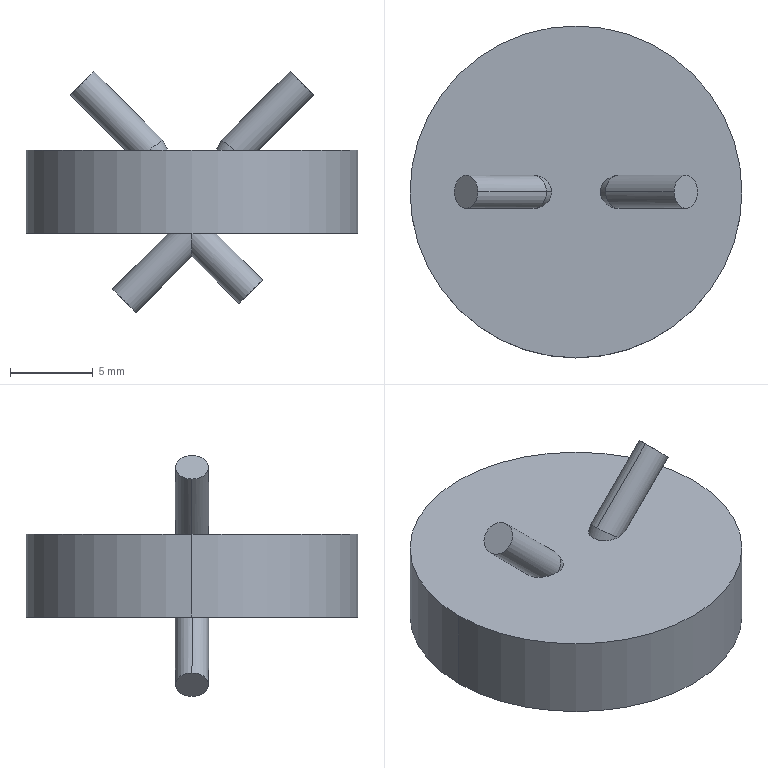Part | SolidWorks | features Sweep 2, Extrusion 1, MirrorPattern 1 | 1 solid | 19 faces | box 20 x 20 x 14.516 mm | volume 1637 mm3 | cylinder 13 | plane 6 | commonest cylinder face diameters 2 x11 20 x2
STEP:
#1=CARTESIAN_POINT('',(1.779,0.,3.098));
#2=VERTEX_POINT('',#1);
#3=CARTESIAN_POINT('',(2.596,1.,2.5));
#4=VERTEX_POINT('',#3);
#5=CARTESIAN_POINT('',(1.779,0.,3.098));
#6=CARTESIAN_POINT('',(1.779,0.5858,3.098));
#7=CARTESIAN_POINT('',(2.118,1.,2.85));
#8=CARTESIAN_POINT('',(2.596,1.,2.5));
#9=(BOUNDED_CURVE()B_SPLINE_CURVE(3,(#5,#6,#7,#8),.UNSPECIFIED.,.F.,.F.)B_SPLINE_CURVE_WITH_KNOTS((4,4),(0.,1.571),.UNSPECIFIED.)CURVE()GEOMETRIC_REPRESENTATION_ITEM()RATIONAL_B_SPLINE_CURVE((1.,0.8047,0.8047,1.))REPRESENTATION_ITEM(''));
#10=EDGE_CURVE('',#2,#4,#9,.T.);
#11=ORIENTED_EDGE('',*,*,#10,.F.);
#12=CARTESIAN_POINT('',(5.912,0.,7.231));
#13=VERTEX_POINT('',#12);
#14=CARTESIAN_POINT('',(1.698,0.,3.016));
#15=DIRECTION('',(0.7071,0.,0.7071));
#16=VECTOR('',#15,1000.);
#17=LINE('',#14,#16);
#18=EDGE_CURVE('',#2,#13,#17,.T.);
#19=ORIENTED_EDGE('',*,*,#18,.T.);
#20=CARTESIAN_POINT('',(7.326,0.,5.816));
#21=VERTEX_POINT('',#20);
#22=CARTESIAN_POINT('',(6.619,0.,6.523));
#23=DIRECTION('',(0.7071,0.,0.7071));
#24=DIRECTION('',(-0.7071,0.,0.7071));
#25=AXIS2_PLACEMENT_3D('',#22,#23,#24);
#26=CIRCLE('',#25,1.);
#27=EDGE_CURVE('',#21,#13,#26,.T.);
#28=ORIENTED_EDGE('',*,*,#27,.F.);
#29=CARTESIAN_POINT('',(4.01,0.,2.5));
#30=VERTEX_POINT('',#29);
#31=CARTESIAN_POINT('',(3.112,0.,1.602));
#32=DIRECTION('',(0.7071,0.,0.7071));
#33=VECTOR('',#32,1000.);
#34=LINE('',#31,#33);
#35=EDGE_CURVE('',#30,#21,#34,.T.);
#36=ORIENTED_EDGE('',*,*,#35,.F.);
#37=CARTESIAN_POINT('',(4.01,0.,2.5));
#38=CARTESIAN_POINT('',(4.01,0.5858,2.5));
#39=CARTESIAN_POINT('',(3.424,1.,2.5));
#40=CARTESIAN_POINT('',(2.596,1.,2.5));
#41=(BOUNDED_CURVE()B_SPLINE_CURVE(3,(#37,#38,#39,#40),.UNSPECIFIED.,.F.,.F.)B_SPLINE_CURVE_WITH_KNOTS((4,4),(0.,1.571),.UNSPECIFIED.)CURVE()GEOMETRIC_REPRESENTATION_ITEM()RATIONAL_B_SPLINE_CURVE((1.,0.8047,0.8047,1.))REPRESENTATION_ITEM(''));
#42=EDGE_CURVE('',#30,#4,#41,.T.);
#43=ORIENTED_EDGE('',*,*,#42,.T.);
#44=EDGE_LOOP('',(#11,#19,#28,#36,#43));
#45=FACE_OUTER_BOUND('',#44,.T.);
#46=CARTESIAN_POINT('',(2.405,0.,2.309));
#47=DIRECTION('',(0.7071,0.,0.7071));
#48=DIRECTION('',(0.7071,0.,-0.7071));
#49=AXIS2_PLACEMENT_3D('',#46,#47,#48);
#50=CYLINDRICAL_SURFACE('',#49,1.);
#51=ADVANCED_FACE('',(#45),#50,.T.);
#52=CARTESIAN_POINT('',(-2.596,-1.,2.5));
#53=VERTEX_POINT('',#52);
#54=CARTESIAN_POINT('',(-1.469,0.,2.5));
#55=VERTEX_POINT('',#54);
#56=CARTESIAN_POINT('',(-2.596,-1.,2.5));
#57=CARTESIAN_POINT('',(-1.936,-1.,2.5));
#58=CARTESIAN_POINT('',(-1.469,-0.5858,2.5));
#59=CARTESIAN_POINT('',(-1.469,0.,2.5));
#60=(BOUNDED_CURVE()B_SPLINE_CURVE(3,(#56,#57,#58,#59),.UNSPECIFIED.,.F.,.T.)B_SPLINE_CURVE_WITH_KNOTS((4,4),(1.571,3.142),.UNSPECIFIED.)CURVE()GEOMETRIC_REPRESENTATION_ITEM()RATIONAL_B_SPLINE_CURVE((1.,0.8047,0.8047,1.))REPRESENTATION_ITEM(''));
#61=EDGE_CURVE('',#53,#55,#60,.T.);
#62=ORIENTED_EDGE('',*,*,#61,.T.);
#63=CARTESIAN_POINT('',(-1.779,0.,3.098));
#64=VERTEX_POINT('',#63);
#65=CARTESIAN_POINT('',(1.012,0.,-2.279));
#66=DIRECTION('',(-0.4608,0.,0.8875));
#67=VECTOR('',#66,1000.);
#68=LINE('',#65,#67);
#69=EDGE_CURVE('',#55,#64,#68,.T.);
#70=ORIENTED_EDGE('',*,*,#69,.T.);
#71=CARTESIAN_POINT('',(-1.779,0.,3.098));
#72=CARTESIAN_POINT('',(-1.779,-0.5858,3.098));
#73=CARTESIAN_POINT('',(-2.118,-1.,2.85));
#74=CARTESIAN_POINT('',(-2.596,-1.,2.5));
#75=(BOUNDED_CURVE()B_SPLINE_CURVE(3,(#71,#72,#73,#74),.UNSPECIFIED.,.F.,.F.)B_SPLINE_CURVE_WITH_KNOTS((4,4),(0.,1.571),.UNSPECIFIED.)CURVE()GEOMETRIC_REPRESENTATION_ITEM()RATIONAL_B_SPLINE_CURVE((1.,0.8047,0.8047,1.))REPRESENTATION_ITEM(''));
#76=EDGE_CURVE('',#64,#53,#75,.T.);
#77=ORIENTED_EDGE('',*,*,#76,.T.);
#78=EDGE_LOOP('',(#62,#70,#77));
#79=FACE_OUTER_BOUND('',#78,.T.);
#80=CARTESIAN_POINT('',(0.1244,0.,-2.74));
#81=DIRECTION('',(-0.4608,0.,0.8875));
#82=DIRECTION('',(0.8875,0.,0.4608));
#83=AXIS2_PLACEMENT_3D('',#80,#81,#82);
#84=CYLINDRICAL_SURFACE('',#83,1.);
#85=ADVANCED_FACE('',(#79),#84,.T.);
#86=CARTESIAN_POINT('',(-2.596,1.,2.5));
#87=VERTEX_POINT('',#86);
#88=CARTESIAN_POINT('',(-4.01,0.,2.5));
#89=VERTEX_POINT('',#88);
#90=CARTESIAN_POINT('',(-2.596,1.,2.5));
#91=CARTESIAN_POINT('',(-3.424,1.,2.5));
#92=CARTESIAN_POINT('',(-4.01,0.5858,2.5));
#93=CARTESIAN_POINT('',(-4.01,0.,2.5));
#94=(BOUNDED_CURVE()B_SPLINE_CURVE(3,(#90,#91,#92,#93),.UNSPECIFIED.,.F.,.T.)B_SPLINE_CURVE_WITH_KNOTS((4,4),(4.712,6.283),.UNSPECIFIED.)CURVE()GEOMETRIC_REPRESENTATION_ITEM()RATIONAL_B_SPLINE_CURVE((1.,0.8047,0.8047,1.))REPRESENTATION_ITEM(''));
#95=EDGE_CURVE('',#87,#89,#94,.T.);
#96=ORIENTED_EDGE('',*,*,#95,.T.);
#97=CARTESIAN_POINT('',(-7.326,0.,5.816));
#98=VERTEX_POINT('',#97);
#99=CARTESIAN_POINT('',(-3.112,0.,1.602));
#100=DIRECTION('',(-0.7071,0.,0.7071));
#101=VECTOR('',#100,1000.);
#102=LINE('',#99,#101);
#103=EDGE_CURVE('',#89,#98,#102,.T.);
#104=ORIENTED_EDGE('',*,*,#103,.T.);
#105=CARTESIAN_POINT('',(-5.912,0.,7.231));
#106=VERTEX_POINT('',#105);
#107=CARTESIAN_POINT('',(-6.619,0.,6.523));
#108=DIRECTION('',(-0.7071,0.,0.7071));
#109=DIRECTION('',(0.7071,0.,0.7071));
#110=AXIS2_PLACEMENT_3D('',#107,#108,#109);
#111=CIRCLE('',#110,1.);
#112=EDGE_CURVE('',#106,#98,#111,.T.);
#113=ORIENTED_EDGE('',*,*,#112,.F.);
#114=CARTESIAN_POINT('',(-1.698,0.,3.016));
#115=DIRECTION('',(-0.7071,0.,0.7071));
#116=VECTOR('',#115,1000.);
#117=LINE('',#114,#116);
#118=EDGE_CURVE('',#64,#106,#117,.T.);
#119=ORIENTED_EDGE('',*,*,#118,.F.);
#120=CARTESIAN_POINT('',(-2.596,1.,2.5));
#121=CARTESIAN_POINT('',(-2.118,1.,2.85));
#122=CARTESIAN_POINT('',(-1.779,0.5858,3.098));
#123=CARTESIAN_POINT('',(-1.779,0.,3.098));
#124=(BOUNDED_CURVE()B_SPLINE_CURVE(3,(#120,#121,#122,#123),.UNSPECIFIED.,.F.,.F.)B_SPLINE_CURVE_WITH_KNOTS((4,4),(4.712,6.283),.UNSPECIFIED.)CURVE()GEOMETRIC_REPRESENTATION_ITEM()RATIONAL_B_SPLINE_CURVE((1.,0.8047,0.8047,1.))REPRESENTATION_ITEM(''));
#125=EDGE_CURVE('',#87,#64,#124,.T.);
#126=ORIENTED_EDGE('',*,*,#125,.F.);
#127=EDGE_LOOP('',(#96,#104,#113,#119,#126));
#128=FACE_OUTER_BOUND('',#127,.T.);
#129=CARTESIAN_POINT('',(-2.405,0.,2.309));
#130=DIRECTION('',(-0.7071,0.,0.7071));
#131=DIRECTION('',(0.7071,0.,0.7071));
#132=AXIS2_PLACEMENT_3D('',#129,#130,#131);
#133=CYLINDRICAL_SURFACE('',#132,1.);
#134=ADVANCED_FACE('',(#128),#133,.T.);
#135=CARTESIAN_POINT('',(-3.371,0.,-7.285));
#136=VERTEX_POINT('',#135);
#137=CARTESIAN_POINT('',(-4.785,0.,-5.871));
#138=VERTEX_POINT('',#137);
#139=CARTESIAN_POINT('',(-4.078,0.,-6.578));
#140=DIRECTION('',(0.7071,0.,0.7071));
#141=DIRECTION('',(0.7071,0.,-0.7071));
#142=AXIS2_PLACEMENT_3D('',#139,#140,#141);
#143=CIRCLE('',#142,1.);
#144=EDGE_CURVE('',#136,#138,#143,.T.);
#145=ORIENTED_EDGE('',*,*,#144,.T.);
#146=CARTESIAN_POINT('',(-1.414,0.,-2.5));
#147=VERTEX_POINT('',#146);
#148=CARTESIAN_POINT('',(-4.785,0.,-5.871));
#149=DIRECTION('',(0.7071,0.,0.7071));
#150=VECTOR('',#149,1000.);
#151=LINE('',#148,#150);
#152=EDGE_CURVE('',#138,#147,#151,.T.);
#153=ORIENTED_EDGE('',*,*,#152,.T.);
#154=CARTESIAN_POINT('',(0.,1.,-2.5));
#155=VERTEX_POINT('',#154);
#156=CARTESIAN_POINT('',(0.,1.,-2.5));
#157=CARTESIAN_POINT('',(-0.8284,1.,-2.5));
#158=CARTESIAN_POINT('',(-1.414,0.5858,-2.5));
#159=CARTESIAN_POINT('',(-1.414,0.,-2.5));
#160=(BOUNDED_CURVE()B_SPLINE_CURVE(3,(#156,#157,#158,#159),.UNSPECIFIED.,.F.,.F.)B_SPLINE_CURVE_WITH_KNOTS((4,4),(1.571,3.142),.UNSPECIFIED.)CURVE()GEOMETRIC_REPRESENTATION_ITEM()RATIONAL_B_SPLINE_CURVE((1.,0.8047,0.8047,1.))REPRESENTATION_ITEM(''));
#161=EDGE_CURVE('',#155,#147,#160,.T.);
#162=ORIENTED_EDGE('',*,*,#161,.F.);
#163=CARTESIAN_POINT('',(0.,0.,-3.914));
#164=VERTEX_POINT('',#163);
#165=CARTESIAN_POINT('',(0.,1.,-2.5));
#166=CARTESIAN_POINT('',(0.,1.,-3.328));
#167=CARTESIAN_POINT('',(0.,0.5858,-3.914));
#168=CARTESIAN_POINT('',(0.,0.,-3.914));
#169=(BOUNDED_CURVE()B_SPLINE_CURVE(3,(#165,#166,#167,#168),.UNSPECIFIED.,.F.,.F.)B_SPLINE_CURVE_WITH_KNOTS((4,4),(1.571,3.142),.UNSPECIFIED.)CURVE()GEOMETRIC_REPRESENTATION_ITEM()RATIONAL_B_SPLINE_CURVE((1.,0.8047,0.8047,1.))REPRESENTATION_ITEM(''));
#170=EDGE_CURVE('',#155,#164,#169,.T.);
#171=ORIENTED_EDGE('',*,*,#170,.T.);
#172=CARTESIAN_POINT('',(-3.371,0.,-7.285));
#173=DIRECTION('',(0.7071,0.,0.7071));
#174=VECTOR('',#173,1000.);
#175=LINE('',#172,#174);
#176=EDGE_CURVE('',#136,#164,#175,.T.);
#177=ORIENTED_EDGE('',*,*,#176,.F.);
#178=EDGE_LOOP('',(#145,#153,#162,#171,#177));
#179=FACE_OUTER_BOUND('',#178,.T.);
#180=CARTESIAN_POINT('',(-4.078,0.,-6.578));
#181=DIRECTION('',(0.7071,0.,0.7071));
#182=DIRECTION('',(0.7071,0.,-0.7071));
#183=AXIS2_PLACEMENT_3D('',#180,#181,#182);
#184=CYLINDRICAL_SURFACE('',#183,1.);
#185=ADVANCED_FACE('',(#179),#184,.T.);
#186=CARTESIAN_POINT('',(1.414,0.,-2.5));
#187=VERTEX_POINT('',#186);
#188=CARTESIAN_POINT('',(1.414,0.,-2.5));
#189=CARTESIAN_POINT('',(1.414,0.5858,-2.5));
#190=CARTESIAN_POINT('',(0.8284,1.,-2.5));
#191=CARTESIAN_POINT('',(0.,1.,-2.5));
#192=(BOUNDED_CURVE()B_SPLINE_CURVE(3,(#188,#189,#190,#191),.UNSPECIFIED.,.F.,.F.)B_SPLINE_CURVE_WITH_KNOTS((4,4),(0.,1.571),.UNSPECIFIED.)CURVE()GEOMETRIC_REPRESENTATION_ITEM()RATIONAL_B_SPLINE_CURVE((1.,0.8047,0.8047,1.))REPRESENTATION_ITEM(''));
#193=EDGE_CURVE('',#187,#155,#192,.T.);
#194=ORIENTED_EDGE('',*,*,#193,.F.);
#195=CARTESIAN_POINT('',(4.243,0.,-5.328));
#196=VERTEX_POINT('',#195);
#197=CARTESIAN_POINT('',(-0.1414,0.,-0.9444));
#198=DIRECTION('',(0.7071,0.,-0.7071));
#199=VECTOR('',#198,1000.);
#200=LINE('',#197,#199);
#201=EDGE_CURVE('',#187,#196,#200,.T.);
#202=ORIENTED_EDGE('',*,*,#201,.T.);
#203=CARTESIAN_POINT('',(2.828,0.,-6.743));
#204=VERTEX_POINT('',#203);
#205=CARTESIAN_POINT('',(3.536,0.,-6.036));
#206=DIRECTION('',(0.7071,0.,-0.7071));
#207=DIRECTION('',(-0.7071,0.,-0.7071));
#208=AXIS2_PLACEMENT_3D('',#205,#206,#207);
#209=CIRCLE('',#208,1.);
#210=EDGE_CURVE('',#204,#196,#209,.T.);
#211=ORIENTED_EDGE('',*,*,#210,.F.);
#212=CARTESIAN_POINT('',(-1.556,0.,-2.359));
#213=DIRECTION('',(0.7071,0.,-0.7071));
#214=VECTOR('',#213,1000.);
#215=LINE('',#212,#214);
#216=EDGE_CURVE('',#164,#204,#215,.T.);
#217=ORIENTED_EDGE('',*,*,#216,.F.);
#218=ORIENTED_EDGE('',*,*,#170,.F.);
#219=EDGE_LOOP('',(#194,#202,#211,#217,#218));
#220=FACE_OUTER_BOUND('',#219,.T.);
#221=CARTESIAN_POINT('',(-0.8485,0.,-1.651));
#222=DIRECTION('',(0.7071,0.,-0.7071));
#223=DIRECTION('',(-0.7071,0.,-0.7071));
#224=AXIS2_PLACEMENT_3D('',#221,#222,#223);
#225=CYLINDRICAL_SURFACE('',#224,1.);
#226=ADVANCED_FACE('',(#220),#225,.T.);
#227=CARTESIAN_POINT('',(10.,0.,2.5));
#228=VERTEX_POINT('',#227);
#229=CARTESIAN_POINT('',(-10.,0.,2.5));
#230=VERTEX_POINT('',#229);
#231=CARTESIAN_POINT('',(0.,0.,2.5));
#232=DIRECTION('',(0.,0.,1.));
#233=DIRECTION('',(1.,0.,0.));
#234=AXIS2_PLACEMENT_3D('',#231,#232,#233);
#235=CIRCLE('',#234,10.);
#236=EDGE_CURVE('',#228,#230,#235,.T.);
#237=ORIENTED_EDGE('',*,*,#236,.F.);
#238=CARTESIAN_POINT('',(10.,0.,-2.5));
#239=VERTEX_POINT('',#238);
#240=CARTESIAN_POINT('',(10.,0.,2.5));
#241=DIRECTION('',(0.,0.,-1.));
#242=VECTOR('',#241,1000.);
#243=LINE('',#240,#242);
#244=EDGE_CURVE('',#228,#239,#243,.T.);
#245=ORIENTED_EDGE('',*,*,#244,.T.);
#246=CARTESIAN_POINT('',(-10.,0.,-2.5));
#247=VERTEX_POINT('',#246);
#248=CARTESIAN_POINT('',(0.,0.,-2.5));
#249=DIRECTION('',(0.,0.,1.));
#250=DIRECTION('',(1.,0.,0.));
#251=AXIS2_PLACEMENT_3D('',#248,#249,#250);
#252=CIRCLE('',#251,10.);
#253=EDGE_CURVE('',#239,#247,#252,.T.);
#254=ORIENTED_EDGE('',*,*,#253,.T.);
#255=CARTESIAN_POINT('',(-10.,0.,2.5));
#256=DIRECTION('',(0.,0.,-1.));
#257=VECTOR('',#256,1000.);
#258=LINE('',#255,#257);
#259=EDGE_CURVE('',#230,#247,#258,.T.);
#260=ORIENTED_EDGE('',*,*,#259,.F.);
#261=EDGE_LOOP('',(#237,#245,#254,#260));
#262=FACE_OUTER_BOUND('',#261,.T.);
#263=CARTESIAN_POINT('',(0.,0.,2.5));
#264=DIRECTION('',(0.,0.,-1.));
#265=DIRECTION('',(-1.,0.,0.));
#266=AXIS2_PLACEMENT_3D('',#263,#264,#265);
#267=CYLINDRICAL_SURFACE('',#266,10.);
#268=ADVANCED_FACE('',(#262),#267,.T.);
#269=ORIENTED_EDGE('',*,*,#244,.F.);
#270=CARTESIAN_POINT('',(0.,0.,2.5));
#271=DIRECTION('',(0.,0.,1.));
#272=DIRECTION('',(1.,0.,0.));
#273=AXIS2_PLACEMENT_3D('',#270,#271,#272);
#274=CIRCLE('',#273,10.);
#275=EDGE_CURVE('',#230,#228,#274,.T.);
#276=ORIENTED_EDGE('',*,*,#275,.F.);
#277=ORIENTED_EDGE('',*,*,#259,.T.);
#278=CARTESIAN_POINT('',(0.,0.,-2.5));
#279=DIRECTION('',(0.,0.,1.));
#280=DIRECTION('',(1.,0.,0.));
#281=AXIS2_PLACEMENT_3D('',#278,#279,#280);
#282=CIRCLE('',#281,10.);
#283=EDGE_CURVE('',#247,#239,#282,.T.);
#284=ORIENTED_EDGE('',*,*,#283,.T.);
#285=EDGE_LOOP('',(#269,#276,#277,#284));
#286=FACE_OUTER_BOUND('',#285,.T.);
#287=CARTESIAN_POINT('',(0.,0.,2.5));
#288=DIRECTION('',(0.,0.,-1.));
#289=DIRECTION('',(-1.,0.,0.));
#290=AXIS2_PLACEMENT_3D('',#287,#288,#289);
#291=CYLINDRICAL_SURFACE('',#290,10.);
#292=ADVANCED_FACE('',(#286),#291,.T.);
#293=CARTESIAN_POINT('',(2.596,-1.,2.5));
#294=VERTEX_POINT('',#293);
#295=CARTESIAN_POINT('',(2.596,-1.,2.5));
#296=CARTESIAN_POINT('',(3.424,-1.,2.5));
#297=CARTESIAN_POINT('',(4.01,-0.5858,2.5));
#298=CARTESIAN_POINT('',(4.01,0.,2.5));
#299=(BOUNDED_CURVE()B_SPLINE_CURVE(3,(#295,#296,#297,#298),.UNSPECIFIED.,.F.,.F.)B_SPLINE_CURVE_WITH_KNOTS((4,4),(4.712,6.283),.UNSPECIFIED.)CURVE()GEOMETRIC_REPRESENTATION_ITEM()RATIONAL_B_SPLINE_CURVE((1.,0.8047,0.8047,1.))REPRESENTATION_ITEM(''));
#300=EDGE_CURVE('',#294,#30,#299,.T.);
#301=ORIENTED_EDGE('',*,*,#300,.F.);
#302=CARTESIAN_POINT('',(2.596,1.,2.5));
#303=CARTESIAN_POINT('',(0.3424,1.,2.5));
#304=CARTESIAN_POINT('',(0.3424,-1.,2.5));
#305=CARTESIAN_POINT('',(2.596,-1.,2.5));
#306=(BOUNDED_CURVE()B_SPLINE_CURVE(3,(#302,#303,#304,#305),.UNSPECIFIED.,.F.,.T.)B_SPLINE_CURVE_WITH_KNOTS((4,4),(1.571,4.712),.UNSPECIFIED.)CURVE()GEOMETRIC_REPRESENTATION_ITEM()RATIONAL_B_SPLINE_CURVE((1.,0.3333,0.3333,1.))REPRESENTATION_ITEM(''));
#307=EDGE_CURVE('',#4,#294,#306,.T.);
#308=ORIENTED_EDGE('',*,*,#307,.F.);
#309=ORIENTED_EDGE('',*,*,#42,.F.);
#310=EDGE_LOOP('',(#301,#308,#309));
#311=FACE_BOUND('',#310,.T.);
#312=ORIENTED_EDGE('',*,*,#95,.F.);
#313=CARTESIAN_POINT('',(-1.469,0.,2.5));
#314=CARTESIAN_POINT('',(-1.469,0.5858,2.5));
#315=CARTESIAN_POINT('',(-1.936,1.,2.5));
#316=CARTESIAN_POINT('',(-2.596,1.,2.5));
#317=(BOUNDED_CURVE()B_SPLINE_CURVE(3,(#313,#314,#315,#316),.UNSPECIFIED.,.F.,.T.)B_SPLINE_CURVE_WITH_KNOTS((4,4),(3.142,4.712),.UNSPECIFIED.)CURVE()GEOMETRIC_REPRESENTATION_ITEM()RATIONAL_B_SPLINE_CURVE((1.,0.8047,0.8047,1.))REPRESENTATION_ITEM(''));
#318=EDGE_CURVE('',#55,#87,#317,.T.);
#319=ORIENTED_EDGE('',*,*,#318,.F.);
#320=ORIENTED_EDGE('',*,*,#61,.F.);
#321=CARTESIAN_POINT('',(-4.01,0.,2.5));
#322=CARTESIAN_POINT('',(-4.01,-0.5858,2.5));
#323=CARTESIAN_POINT('',(-3.424,-1.,2.5));
#324=CARTESIAN_POINT('',(-2.596,-1.,2.5));
#325=(BOUNDED_CURVE()B_SPLINE_CURVE(3,(#321,#322,#323,#324),.UNSPECIFIED.,.F.,.F.)B_SPLINE_CURVE_WITH_KNOTS((4,4),(0.,1.571),.UNSPECIFIED.)CURVE()GEOMETRIC_REPRESENTATION_ITEM()RATIONAL_B_SPLINE_CURVE((1.,0.8047,0.8047,1.))REPRESENTATION_ITEM(''));
#326=EDGE_CURVE('',#89,#53,#325,.T.);
#327=ORIENTED_EDGE('',*,*,#326,.F.);
#328=EDGE_LOOP('',(#312,#319,#320,#327));
#329=FACE_BOUND('',#328,.T.);
#330=ORIENTED_EDGE('',*,*,#275,.T.);
#331=ORIENTED_EDGE('',*,*,#236,.T.);
#332=EDGE_LOOP('',(#330,#331));
#333=FACE_OUTER_BOUND('',#332,.T.);
#334=CARTESIAN_POINT('',(0.,0.,2.5));
#335=DIRECTION('',(0.,0.,1.));
#336=DIRECTION('',(1.,0.,0.));
#337=AXIS2_PLACEMENT_3D('',#334,#335,#336);
#338=PLANE('',#337);
#339=ADVANCED_FACE('',(#311,#329,#333),#338,.T.);
#340=ORIENTED_EDGE('',*,*,#161,.T.);
#341=CARTESIAN_POINT('',(0.,-1.,-2.5));
#342=VERTEX_POINT('',#341);
#343=CARTESIAN_POINT('',(-1.414,0.,-2.5));
#344=CARTESIAN_POINT('',(-1.414,-0.5858,-2.5));
#345=CARTESIAN_POINT('',(-0.8284,-1.,-2.5));
#346=CARTESIAN_POINT('',(0.,-1.,-2.5));
#347=(BOUNDED_CURVE()B_SPLINE_CURVE(3,(#343,#344,#345,#346),.UNSPECIFIED.,.F.,.F.)B_SPLINE_CURVE_WITH_KNOTS((4,4),(3.142,4.712),.UNSPECIFIED.)CURVE()GEOMETRIC_REPRESENTATION_ITEM()RATIONAL_B_SPLINE_CURVE((1.,0.8047,0.8047,1.))REPRESENTATION_ITEM(''));
#348=EDGE_CURVE('',#147,#342,#347,.T.);
#349=ORIENTED_EDGE('',*,*,#348,.T.);
#350=CARTESIAN_POINT('',(0.,-1.,-2.5));
#351=CARTESIAN_POINT('',(0.8284,-1.,-2.5));
#352=CARTESIAN_POINT('',(1.414,-0.5858,-2.5));
#353=CARTESIAN_POINT('',(1.414,0.,-2.5));
#354=(BOUNDED_CURVE()B_SPLINE_CURVE(3,(#350,#351,#352,#353),.UNSPECIFIED.,.F.,.F.)B_SPLINE_CURVE_WITH_KNOTS((4,4),(4.712,6.283),.UNSPECIFIED.)CURVE()GEOMETRIC_REPRESENTATION_ITEM()RATIONAL_B_SPLINE_CURVE((1.,0.8047,0.8047,1.))REPRESENTATION_ITEM(''));
#355=EDGE_CURVE('',#342,#187,#354,.T.);
#356=ORIENTED_EDGE('',*,*,#355,.T.);
#357=ORIENTED_EDGE('',*,*,#193,.T.);
#358=EDGE_LOOP('',(#340,#349,#356,#357));
#359=FACE_BOUND('',#358,.T.);
#360=ORIENTED_EDGE('',*,*,#283,.F.);
#361=ORIENTED_EDGE('',*,*,#253,.F.);
#362=EDGE_LOOP('',(#360,#361));
#363=FACE_OUTER_BOUND('',#362,.T.);
#364=CARTESIAN_POINT('',(0.,0.,-2.5));
#365=DIRECTION('',(0.,0.,1.));
#366=DIRECTION('',(1.,0.,0.));
#367=AXIS2_PLACEMENT_3D('',#364,#365,#366);
#368=PLANE('',#367);
#369=ADVANCED_FACE('',(#359,#363),#368,.F.);
#370=ORIENTED_EDGE('',*,*,#201,.F.);
#371=ORIENTED_EDGE('',*,*,#355,.F.);
#372=CARTESIAN_POINT('',(0.,0.,-3.914));
#373=CARTESIAN_POINT('',(0.,-0.5858,-3.914));
#374=CARTESIAN_POINT('',(0.,-1.,-3.328));
#375=CARTESIAN_POINT('',(0.,-1.,-2.5));
#376=(BOUNDED_CURVE()B_SPLINE_CURVE(3,(#372,#373,#374,#375),.UNSPECIFIED.,.F.,.F.)B_SPLINE_CURVE_WITH_KNOTS((4,4),(3.142,4.712),.UNSPECIFIED.)CURVE()GEOMETRIC_REPRESENTATION_ITEM()RATIONAL_B_SPLINE_CURVE((1.,0.8047,0.8047,1.))REPRESENTATION_ITEM(''));
#377=EDGE_CURVE('',#164,#342,#376,.T.);
#378=ORIENTED_EDGE('',*,*,#377,.F.);
#379=ORIENTED_EDGE('',*,*,#216,.T.);
#380=CARTESIAN_POINT('',(3.536,0.,-6.036));
#381=DIRECTION('',(0.7071,0.,-0.7071));
#382=DIRECTION('',(-0.7071,0.,-0.7071));
#383=AXIS2_PLACEMENT_3D('',#380,#381,#382);
#384=CIRCLE('',#383,1.);
#385=EDGE_CURVE('',#196,#204,#384,.T.);
#386=ORIENTED_EDGE('',*,*,#385,.F.);
#387=EDGE_LOOP('',(#370,#371,#378,#379,#386));
#388=FACE_OUTER_BOUND('',#387,.T.);
#389=CARTESIAN_POINT('',(-0.8485,0.,-1.651));
#390=DIRECTION('',(0.7071,0.,-0.7071));
#391=DIRECTION('',(-0.7071,0.,-0.7071));
#392=AXIS2_PLACEMENT_3D('',#389,#390,#391);
#393=CYLINDRICAL_SURFACE('',#392,1.);
#394=ADVANCED_FACE('',(#388),#393,.T.);
#395=ORIENTED_EDGE('',*,*,#152,.F.);
#396=CARTESIAN_POINT('',(-4.078,0.,-6.578));
#397=DIRECTION('',(0.7071,0.,0.7071));
#398=DIRECTION('',(0.7071,0.,-0.7071));
#399=AXIS2_PLACEMENT_3D('',#396,#397,#398);
#400=CIRCLE('',#399,1.);
#401=EDGE_CURVE('',#138,#136,#400,.T.);
#402=ORIENTED_EDGE('',*,*,#401,.T.);
#403=ORIENTED_EDGE('',*,*,#176,.T.);
#404=ORIENTED_EDGE('',*,*,#377,.T.);
#405=ORIENTED_EDGE('',*,*,#348,.F.);
#406=EDGE_LOOP('',(#395,#402,#403,#404,#405));
#407=FACE_OUTER_BOUND('',#406,.T.);
#408=CARTESIAN_POINT('',(-4.078,0.,-6.578));
#409=DIRECTION('',(0.7071,0.,0.7071));
#410=DIRECTION('',(0.7071,0.,-0.7071));
#411=AXIS2_PLACEMENT_3D('',#408,#409,#410);
#412=CYLINDRICAL_SURFACE('',#411,1.);
#413=ADVANCED_FACE('',(#407),#412,.T.);
#414=ORIENTED_EDGE('',*,*,#144,.F.);
#415=ORIENTED_EDGE('',*,*,#401,.F.);
#416=EDGE_LOOP('',(#414,#415));
#417=FACE_OUTER_BOUND('',#416,.T.);
#418=CARTESIAN_POINT('',(-4.078,0.,-6.578));
#419=DIRECTION('',(0.7071,0.,0.7071));
#420=DIRECTION('',(0.7071,0.,-0.7071));
#421=AXIS2_PLACEMENT_3D('',#418,#419,#420);
#422=PLANE('',#421);
#423=ADVANCED_FACE('',(#417),#422,.F.);
#424=ORIENTED_EDGE('',*,*,#210,.T.);
#425=ORIENTED_EDGE('',*,*,#385,.T.);
#426=EDGE_LOOP('',(#424,#425));
#427=FACE_OUTER_BOUND('',#426,.T.);
#428=CARTESIAN_POINT('',(3.536,0.,-6.036));
#429=DIRECTION('',(0.7071,0.,-0.7071));
#430=DIRECTION('',(-0.7071,0.,-0.7071));
#431=AXIS2_PLACEMENT_3D('',#428,#429,#430);
#432=PLANE('',#431);
#433=ADVANCED_FACE('',(#427),#432,.T.);
#434=ORIENTED_EDGE('',*,*,#69,.F.);
#435=ORIENTED_EDGE('',*,*,#318,.T.);
#436=ORIENTED_EDGE('',*,*,#125,.T.);
#437=EDGE_LOOP('',(#434,#435,#436));
#438=FACE_OUTER_BOUND('',#437,.T.);
#439=CARTESIAN_POINT('',(0.1244,0.,-2.74));
#440=DIRECTION('',(-0.4608,0.,0.8875));
#441=DIRECTION('',(0.8875,0.,0.4608));
#442=AXIS2_PLACEMENT_3D('',#439,#440,#441);
#443=CYLINDRICAL_SURFACE('',#442,1.);
#444=ADVANCED_FACE('',(#438),#443,.T.);
#445=ORIENTED_EDGE('',*,*,#103,.F.);
#446=ORIENTED_EDGE('',*,*,#326,.T.);
#447=ORIENTED_EDGE('',*,*,#76,.F.);
#448=ORIENTED_EDGE('',*,*,#118,.T.);
#449=CARTESIAN_POINT('',(-6.619,0.,6.523));
#450=DIRECTION('',(-0.7071,0.,0.7071));
#451=DIRECTION('',(0.7071,0.,0.7071));
#452=AXIS2_PLACEMENT_3D('',#449,#450,#451);
#453=CIRCLE('',#452,1.);
#454=EDGE_CURVE('',#98,#106,#453,.T.);
#455=ORIENTED_EDGE('',*,*,#454,.F.);
#456=EDGE_LOOP('',(#445,#446,#447,#448,#455));
#457=FACE_OUTER_BOUND('',#456,.T.);
#458=CARTESIAN_POINT('',(-2.405,0.,2.309));
#459=DIRECTION('',(-0.7071,0.,0.7071));
#460=DIRECTION('',(0.7071,0.,0.7071));
#461=AXIS2_PLACEMENT_3D('',#458,#459,#460);
#462=CYLINDRICAL_SURFACE('',#461,1.);
#463=ADVANCED_FACE('',(#457),#462,.T.);
#464=ORIENTED_EDGE('',*,*,#112,.T.);
#465=ORIENTED_EDGE('',*,*,#454,.T.);
#466=EDGE_LOOP('',(#464,#465));
#467=FACE_OUTER_BOUND('',#466,.T.);
#468=CARTESIAN_POINT('',(-6.619,0.,6.523));
#469=DIRECTION('',(-0.7071,0.,0.7071));
#470=DIRECTION('',(0.7071,0.,0.7071));
#471=AXIS2_PLACEMENT_3D('',#468,#469,#470);
#472=PLANE('',#471);
#473=ADVANCED_FACE('',(#467),#472,.T.);
#474=CARTESIAN_POINT('',(2.596,-1.,2.5));
#475=CARTESIAN_POINT('',(2.118,-1.,2.85));
#476=CARTESIAN_POINT('',(1.779,-0.5858,3.098));
#477=CARTESIAN_POINT('',(1.779,0.,3.098));
#478=(BOUNDED_CURVE()B_SPLINE_CURVE(3,(#474,#475,#476,#477),.UNSPECIFIED.,.F.,.F.)B_SPLINE_CURVE_WITH_KNOTS((4,4),(4.712,6.283),.UNSPECIFIED.)CURVE()GEOMETRIC_REPRESENTATION_ITEM()RATIONAL_B_SPLINE_CURVE((1.,0.8047,0.8047,1.))REPRESENTATION_ITEM(''));
#479=EDGE_CURVE('',#294,#2,#478,.T.);
#480=ORIENTED_EDGE('',*,*,#479,.T.);
#481=ORIENTED_EDGE('',*,*,#10,.T.);
#482=ORIENTED_EDGE('',*,*,#307,.T.);
#483=EDGE_LOOP('',(#480,#481,#482));
#484=FACE_OUTER_BOUND('',#483,.T.);
#485=CARTESIAN_POINT('',(-0.1244,0.,-2.74));
#486=DIRECTION('',(0.4608,0.,0.8875));
#487=DIRECTION('',(0.8875,0.,-0.4608));
#488=AXIS2_PLACEMENT_3D('',#485,#486,#487);
#489=CYLINDRICAL_SURFACE('',#488,1.);
#490=ADVANCED_FACE('',(#484),#489,.T.);
#491=ORIENTED_EDGE('',*,*,#18,.F.);
#492=ORIENTED_EDGE('',*,*,#479,.F.);
#493=ORIENTED_EDGE('',*,*,#300,.T.);
#494=ORIENTED_EDGE('',*,*,#35,.T.);
#495=CARTESIAN_POINT('',(6.619,0.,6.523));
#496=DIRECTION('',(0.7071,0.,0.7071));
#497=DIRECTION('',(-0.7071,0.,0.7071));
#498=AXIS2_PLACEMENT_3D('',#495,#496,#497);
#499=CIRCLE('',#498,1.);
#500=EDGE_CURVE('',#13,#21,#499,.T.);
#501=ORIENTED_EDGE('',*,*,#500,.F.);
#502=EDGE_LOOP('',(#491,#492,#493,#494,#501));
#503=FACE_OUTER_BOUND('',#502,.T.);
#504=CARTESIAN_POINT('',(2.405,0.,2.309));
#505=DIRECTION('',(0.7071,0.,0.7071));
#506=DIRECTION('',(0.7071,0.,-0.7071));
#507=AXIS2_PLACEMENT_3D('',#504,#505,#506);
#508=CYLINDRICAL_SURFACE('',#507,1.);
#509=ADVANCED_FACE('',(#503),#508,.T.);
#510=ORIENTED_EDGE('',*,*,#27,.T.);
#511=ORIENTED_EDGE('',*,*,#500,.T.);
#512=EDGE_LOOP('',(#510,#511));
#513=FACE_OUTER_BOUND('',#512,.T.);
#514=CARTESIAN_POINT('',(6.619,0.,6.523));
#515=DIRECTION('',(0.7071,0.,0.7071));
#516=DIRECTION('',(-0.7071,0.,0.7071));
#517=AXIS2_PLACEMENT_3D('',#514,#515,#516);
#518=PLANE('',#517);
#519=ADVANCED_FACE('',(#513),#518,.T.);
#520=CLOSED_SHELL('',(#51,#85,#134,#185,#226,#268,#292,#339,#369,#394,#413,#423,#433,#444,#463,#473,#490,#509,#519));
#521=MANIFOLD_SOLID_BREP('',#520);
#522=CARTESIAN_POINT('',(0.,0.,0.));
#523=DIRECTION('',(0.,0.,1.));
#524=DIRECTION('',(1.,0.,0.));
#525=AXIS2_PLACEMENT_3D('',#522,#523,#524);
#526=(LENGTH_UNIT()NAMED_UNIT(*)SI_UNIT(.MILLI.,.METRE.));
#527=UNCERTAINTY_MEASURE_WITH_UNIT(LENGTH_MEASURE(0.00001),#526,'','');
#528=(NAMED_UNIT(*)PLANE_ANGLE_UNIT()SI_UNIT($,.RADIAN.));
#529=(NAMED_UNIT(*)SI_UNIT($,.STERADIAN.)SOLID_ANGLE_UNIT());
#530=(GEOMETRIC_REPRESENTATION_CONTEXT(3)GLOBAL_UNCERTAINTY_ASSIGNED_CONTEXT((#527))GLOBAL_UNIT_ASSIGNED_CONTEXT((#526,#528,#529))REPRESENTATION_CONTEXT('',''));
#531=ADVANCED_BREP_SHAPE_REPRESENTATION('',(#521,#525),#530);